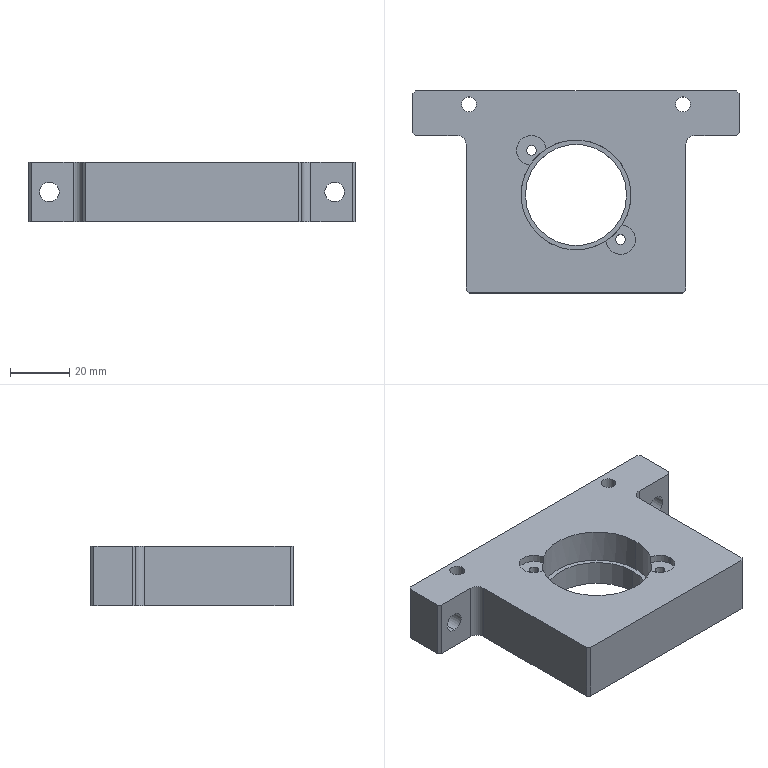Part | STEP file | Bearing mounting plate A | 1 solid | 40 faces | box 110 x 68 x 20 mm | volume 88933 mm3 | cylinder 21 | plane 19 | commonest cylinder face diameters 3.3 x4 5 x4 6.6 x4 10 x3 6 x2 34 x2